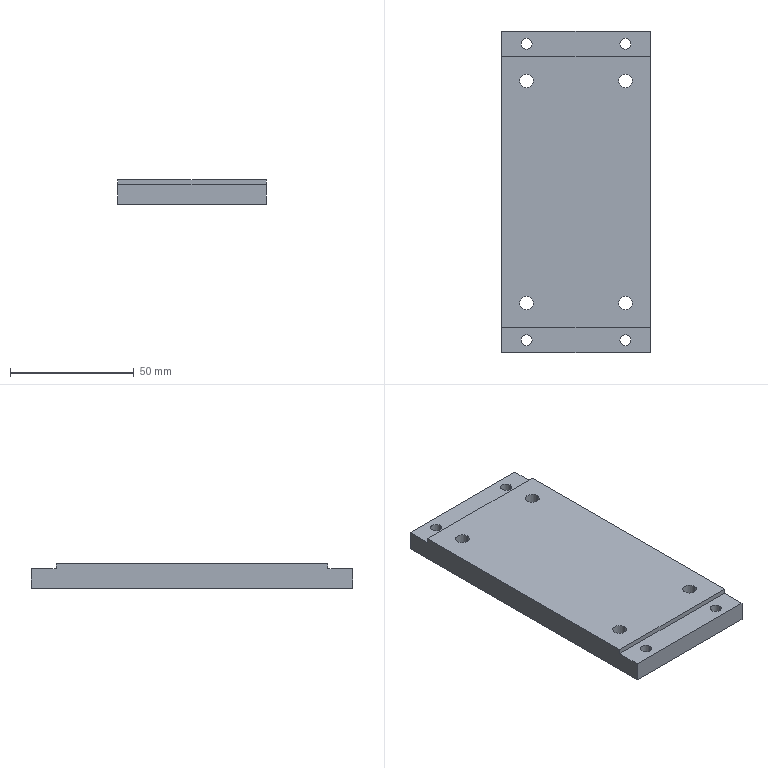Part | SolidWorks | features HoleWzd 2, Extrusion 1, ICE 1 | 1 solid | 38 faces | box 60 x 130 x 10 mm | volume 73508 mm3 | cylinder 24 | plane 14 | commonest cylinder face diameters 4.5 x8 5.5 x8 8 x8
STEP:
#1=CARTESIAN_POINT('',(17.25,45.,0.));
#2=VERTEX_POINT('',#1);
#3=CARTESIAN_POINT('',(22.75,45.,0.));
#4=VERTEX_POINT('',#3);
#5=CARTESIAN_POINT('',(20.,45.,0.));
#6=DIRECTION('',(0.,0.,1.));
#7=DIRECTION('',(1.,0.,0.));
#8=AXIS2_PLACEMENT_3D('',#5,#6,#7);
#9=CIRCLE('',#8,2.75);
#10=EDGE_CURVE('',#2,#4,#9,.T.);
#11=ORIENTED_EDGE('',*,*,#10,.F.);
#12=CARTESIAN_POINT('',(17.25,45.,10.));
#13=VERTEX_POINT('',#12);
#14=CARTESIAN_POINT('',(17.25,45.,10.));
#15=DIRECTION('',(0.,0.,1.));
#16=VECTOR('',#15,1000.);
#17=LINE('',#14,#16);
#18=EDGE_CURVE('',#2,#13,#17,.T.);
#19=ORIENTED_EDGE('',*,*,#18,.T.);
#20=CARTESIAN_POINT('',(22.75,45.,10.));
#21=VERTEX_POINT('',#20);
#22=CARTESIAN_POINT('',(20.,45.,10.));
#23=DIRECTION('',(0.,0.,1.));
#24=DIRECTION('',(1.,0.,0.));
#25=AXIS2_PLACEMENT_3D('',#22,#23,#24);
#26=CIRCLE('',#25,2.75);
#27=EDGE_CURVE('',#13,#21,#26,.T.);
#28=ORIENTED_EDGE('',*,*,#27,.T.);
#29=CARTESIAN_POINT('',(22.75,45.,10.));
#30=DIRECTION('',(0.,0.,1.));
#31=VECTOR('',#30,1000.);
#32=LINE('',#29,#31);
#33=EDGE_CURVE('',#4,#21,#32,.T.);
#34=ORIENTED_EDGE('',*,*,#33,.F.);
#35=EDGE_LOOP('',(#11,#19,#28,#34));
#36=FACE_OUTER_BOUND('',#35,.T.);
#37=CARTESIAN_POINT('',(20.,45.,10.));
#38=DIRECTION('',(0.,0.,1.));
#39=DIRECTION('',(1.,0.,0.));
#40=AXIS2_PLACEMENT_3D('',#37,#38,#39);
#41=CYLINDRICAL_SURFACE('',#40,2.75);
#42=ADVANCED_FACE('',(#36),#41,.F.);
#43=CARTESIAN_POINT('',(17.25,-45.,0.));
#44=VERTEX_POINT('',#43);
#45=CARTESIAN_POINT('',(22.75,-45.,0.));
#46=VERTEX_POINT('',#45);
#47=CARTESIAN_POINT('',(20.,-45.,0.));
#48=DIRECTION('',(0.,0.,1.));
#49=DIRECTION('',(1.,0.,0.));
#50=AXIS2_PLACEMENT_3D('',#47,#48,#49);
#51=CIRCLE('',#50,2.75);
#52=EDGE_CURVE('',#44,#46,#51,.T.);
#53=ORIENTED_EDGE('',*,*,#52,.F.);
#54=CARTESIAN_POINT('',(17.25,-45.,10.));
#55=VERTEX_POINT('',#54);
#56=CARTESIAN_POINT('',(17.25,-45.,10.));
#57=DIRECTION('',(0.,0.,1.));
#58=VECTOR('',#57,1000.);
#59=LINE('',#56,#58);
#60=EDGE_CURVE('',#44,#55,#59,.T.);
#61=ORIENTED_EDGE('',*,*,#60,.T.);
#62=CARTESIAN_POINT('',(22.75,-45.,10.));
#63=VERTEX_POINT('',#62);
#64=CARTESIAN_POINT('',(20.,-45.,10.));
#65=DIRECTION('',(0.,0.,1.));
#66=DIRECTION('',(1.,0.,0.));
#67=AXIS2_PLACEMENT_3D('',#64,#65,#66);
#68=CIRCLE('',#67,2.75);
#69=EDGE_CURVE('',#55,#63,#68,.T.);
#70=ORIENTED_EDGE('',*,*,#69,.T.);
#71=CARTESIAN_POINT('',(22.75,-45.,10.));
#72=DIRECTION('',(0.,0.,1.));
#73=VECTOR('',#72,1000.);
#74=LINE('',#71,#73);
#75=EDGE_CURVE('',#46,#63,#74,.T.);
#76=ORIENTED_EDGE('',*,*,#75,.F.);
#77=EDGE_LOOP('',(#53,#61,#70,#76));
#78=FACE_OUTER_BOUND('',#77,.T.);
#79=CARTESIAN_POINT('',(20.,-45.,10.));
#80=DIRECTION('',(0.,0.,1.));
#81=DIRECTION('',(1.,0.,0.));
#82=AXIS2_PLACEMENT_3D('',#79,#80,#81);
#83=CYLINDRICAL_SURFACE('',#82,2.75);
#84=ADVANCED_FACE('',(#78),#83,.F.);
#85=CARTESIAN_POINT('',(-22.75,45.,0.));
#86=VERTEX_POINT('',#85);
#87=CARTESIAN_POINT('',(-17.25,45.,0.));
#88=VERTEX_POINT('',#87);
#89=CARTESIAN_POINT('',(-20.,45.,0.));
#90=DIRECTION('',(0.,0.,1.));
#91=DIRECTION('',(1.,0.,0.));
#92=AXIS2_PLACEMENT_3D('',#89,#90,#91);
#93=CIRCLE('',#92,2.75);
#94=EDGE_CURVE('',#86,#88,#93,.T.);
#95=ORIENTED_EDGE('',*,*,#94,.F.);
#96=CARTESIAN_POINT('',(-22.75,45.,10.));
#97=VERTEX_POINT('',#96);
#98=CARTESIAN_POINT('',(-22.75,45.,10.));
#99=DIRECTION('',(0.,0.,1.));
#100=VECTOR('',#99,1000.);
#101=LINE('',#98,#100);
#102=EDGE_CURVE('',#86,#97,#101,.T.);
#103=ORIENTED_EDGE('',*,*,#102,.T.);
#104=CARTESIAN_POINT('',(-17.25,45.,10.));
#105=VERTEX_POINT('',#104);
#106=CARTESIAN_POINT('',(-20.,45.,10.));
#107=DIRECTION('',(0.,0.,1.));
#108=DIRECTION('',(1.,0.,0.));
#109=AXIS2_PLACEMENT_3D('',#106,#107,#108);
#110=CIRCLE('',#109,2.75);
#111=EDGE_CURVE('',#97,#105,#110,.T.);
#112=ORIENTED_EDGE('',*,*,#111,.T.);
#113=CARTESIAN_POINT('',(-17.25,45.,10.));
#114=DIRECTION('',(0.,0.,1.));
#115=VECTOR('',#114,1000.);
#116=LINE('',#113,#115);
#117=EDGE_CURVE('',#88,#105,#116,.T.);
#118=ORIENTED_EDGE('',*,*,#117,.F.);
#119=EDGE_LOOP('',(#95,#103,#112,#118));
#120=FACE_OUTER_BOUND('',#119,.T.);
#121=CARTESIAN_POINT('',(-20.,45.,10.));
#122=DIRECTION('',(0.,0.,1.));
#123=DIRECTION('',(1.,0.,0.));
#124=AXIS2_PLACEMENT_3D('',#121,#122,#123);
#125=CYLINDRICAL_SURFACE('',#124,2.75);
#126=ADVANCED_FACE('',(#120),#125,.F.);
#127=CARTESIAN_POINT('',(-22.75,-45.,0.));
#128=VERTEX_POINT('',#127);
#129=CARTESIAN_POINT('',(-17.25,-45.,0.));
#130=VERTEX_POINT('',#129);
#131=CARTESIAN_POINT('',(-20.,-45.,0.));
#132=DIRECTION('',(0.,0.,1.));
#133=DIRECTION('',(1.,0.,0.));
#134=AXIS2_PLACEMENT_3D('',#131,#132,#133);
#135=CIRCLE('',#134,2.75);
#136=EDGE_CURVE('',#128,#130,#135,.T.);
#137=ORIENTED_EDGE('',*,*,#136,.F.);
#138=CARTESIAN_POINT('',(-22.75,-45.,10.));
#139=VERTEX_POINT('',#138);
#140=CARTESIAN_POINT('',(-22.75,-45.,10.));
#141=DIRECTION('',(0.,0.,1.));
#142=VECTOR('',#141,1000.);
#143=LINE('',#140,#142);
#144=EDGE_CURVE('',#128,#139,#143,.T.);
#145=ORIENTED_EDGE('',*,*,#144,.T.);
#146=CARTESIAN_POINT('',(-17.25,-45.,10.));
#147=VERTEX_POINT('',#146);
#148=CARTESIAN_POINT('',(-20.,-45.,10.));
#149=DIRECTION('',(0.,0.,1.));
#150=DIRECTION('',(1.,0.,0.));
#151=AXIS2_PLACEMENT_3D('',#148,#149,#150);
#152=CIRCLE('',#151,2.75);
#153=EDGE_CURVE('',#139,#147,#152,.T.);
#154=ORIENTED_EDGE('',*,*,#153,.T.);
#155=CARTESIAN_POINT('',(-17.25,-45.,10.));
#156=DIRECTION('',(0.,0.,1.));
#157=VECTOR('',#156,1000.);
#158=LINE('',#155,#157);
#159=EDGE_CURVE('',#130,#147,#158,.T.);
#160=ORIENTED_EDGE('',*,*,#159,.F.);
#161=EDGE_LOOP('',(#137,#145,#154,#160));
#162=FACE_OUTER_BOUND('',#161,.T.);
#163=CARTESIAN_POINT('',(-20.,-45.,10.));
#164=DIRECTION('',(0.,0.,1.));
#165=DIRECTION('',(1.,0.,0.));
#166=AXIS2_PLACEMENT_3D('',#163,#164,#165);
#167=CYLINDRICAL_SURFACE('',#166,2.75);
#168=ADVANCED_FACE('',(#162),#167,.F.);
#169=CARTESIAN_POINT('',(-16.,-60.,4.6));
#170=VERTEX_POINT('',#169);
#171=CARTESIAN_POINT('',(-24.,-60.,4.6));
#172=VERTEX_POINT('',#171);
#173=CARTESIAN_POINT('',(-20.,-60.,4.6));
#174=DIRECTION('',(0.,0.,-1.));
#175=DIRECTION('',(-1.,0.,0.));
#176=AXIS2_PLACEMENT_3D('',#173,#174,#175);
#177=CIRCLE('',#176,4.);
#178=EDGE_CURVE('',#170,#172,#177,.T.);
#179=ORIENTED_EDGE('',*,*,#178,.F.);
#180=CARTESIAN_POINT('',(-16.,-60.,0.));
#181=VERTEX_POINT('',#180);
#182=CARTESIAN_POINT('',(-16.,-60.,0.));
#183=DIRECTION('',(0.,0.,-1.));
#184=VECTOR('',#183,1000.);
#185=LINE('',#182,#184);
#186=EDGE_CURVE('',#170,#181,#185,.T.);
#187=ORIENTED_EDGE('',*,*,#186,.T.);
#188=CARTESIAN_POINT('',(-24.,-60.,0.));
#189=VERTEX_POINT('',#188);
#190=CARTESIAN_POINT('',(-20.,-60.,0.));
#191=DIRECTION('',(0.,0.,-1.));
#192=DIRECTION('',(-1.,0.,0.));
#193=AXIS2_PLACEMENT_3D('',#190,#191,#192);
#194=CIRCLE('',#193,4.);
#195=EDGE_CURVE('',#181,#189,#194,.T.);
#196=ORIENTED_EDGE('',*,*,#195,.T.);
#197=CARTESIAN_POINT('',(-24.,-60.,0.));
#198=DIRECTION('',(0.,0.,-1.));
#199=VECTOR('',#198,1000.);
#200=LINE('',#197,#199);
#201=EDGE_CURVE('',#172,#189,#200,.T.);
#202=ORIENTED_EDGE('',*,*,#201,.F.);
#203=EDGE_LOOP('',(#179,#187,#196,#202));
#204=FACE_OUTER_BOUND('',#203,.T.);
#205=CARTESIAN_POINT('',(-20.,-60.,0.));
#206=DIRECTION('',(0.,0.,-1.));
#207=DIRECTION('',(-1.,0.,0.));
#208=AXIS2_PLACEMENT_3D('',#205,#206,#207);
#209=CYLINDRICAL_SURFACE('',#208,4.);
#210=ADVANCED_FACE('',(#204),#209,.F.);
#211=CARTESIAN_POINT('',(-22.25,-60.,8.));
#212=VERTEX_POINT('',#211);
#213=CARTESIAN_POINT('',(-17.75,-60.,8.));
#214=VERTEX_POINT('',#213);
#215=CARTESIAN_POINT('',(-20.,-60.,8.));
#216=DIRECTION('',(0.,0.,1.));
#217=DIRECTION('',(1.,0.,0.));
#218=AXIS2_PLACEMENT_3D('',#215,#216,#217);
#219=CIRCLE('',#218,2.25);
#220=EDGE_CURVE('',#212,#214,#219,.T.);
#221=ORIENTED_EDGE('',*,*,#220,.T.);
#222=CARTESIAN_POINT('',(-17.75,-60.,4.6));
#223=VERTEX_POINT('',#222);
#224=CARTESIAN_POINT('',(-17.75,-60.,0.));
#225=DIRECTION('',(0.,0.,-1.));
#226=VECTOR('',#225,1000.);
#227=LINE('',#224,#226);
#228=EDGE_CURVE('',#214,#223,#227,.T.);
#229=ORIENTED_EDGE('',*,*,#228,.T.);
#230=CARTESIAN_POINT('',(-22.25,-60.,4.6));
#231=VERTEX_POINT('',#230);
#232=CARTESIAN_POINT('',(-20.,-60.,4.6));
#233=DIRECTION('',(0.,0.,-1.));
#234=DIRECTION('',(-1.,0.,0.));
#235=AXIS2_PLACEMENT_3D('',#232,#233,#234);
#236=CIRCLE('',#235,2.25);
#237=EDGE_CURVE('',#223,#231,#236,.T.);
#238=ORIENTED_EDGE('',*,*,#237,.T.);
#239=CARTESIAN_POINT('',(-22.25,-60.,0.));
#240=DIRECTION('',(0.,0.,-1.));
#241=VECTOR('',#240,1000.);
#242=LINE('',#239,#241);
#243=EDGE_CURVE('',#212,#231,#242,.T.);
#244=ORIENTED_EDGE('',*,*,#243,.F.);
#245=EDGE_LOOP('',(#221,#229,#238,#244));
#246=FACE_OUTER_BOUND('',#245,.T.);
#247=CARTESIAN_POINT('',(-20.,-60.,0.));
#248=DIRECTION('',(0.,0.,-1.));
#249=DIRECTION('',(-1.,0.,0.));
#250=AXIS2_PLACEMENT_3D('',#247,#248,#249);
#251=CYLINDRICAL_SURFACE('',#250,2.25);
#252=ADVANCED_FACE('',(#246),#251,.F.);
#253=CARTESIAN_POINT('',(24.,-60.,4.6));
#254=VERTEX_POINT('',#253);
#255=CARTESIAN_POINT('',(16.,-60.,4.6));
#256=VERTEX_POINT('',#255);
#257=CARTESIAN_POINT('',(20.,-60.,4.6));
#258=DIRECTION('',(0.,0.,-1.));
#259=DIRECTION('',(-1.,0.,0.));
#260=AXIS2_PLACEMENT_3D('',#257,#258,#259);
#261=CIRCLE('',#260,4.);
#262=EDGE_CURVE('',#254,#256,#261,.T.);
#263=ORIENTED_EDGE('',*,*,#262,.F.);
#264=CARTESIAN_POINT('',(24.,-60.,0.));
#265=VERTEX_POINT('',#264);
#266=CARTESIAN_POINT('',(24.,-60.,0.));
#267=DIRECTION('',(0.,0.,-1.));
#268=VECTOR('',#267,1000.);
#269=LINE('',#266,#268);
#270=EDGE_CURVE('',#254,#265,#269,.T.);
#271=ORIENTED_EDGE('',*,*,#270,.T.);
#272=CARTESIAN_POINT('',(16.,-60.,0.));
#273=VERTEX_POINT('',#272);
#274=CARTESIAN_POINT('',(20.,-60.,0.));
#275=DIRECTION('',(0.,0.,-1.));
#276=DIRECTION('',(-1.,0.,0.));
#277=AXIS2_PLACEMENT_3D('',#274,#275,#276);
#278=CIRCLE('',#277,4.);
#279=EDGE_CURVE('',#265,#273,#278,.T.);
#280=ORIENTED_EDGE('',*,*,#279,.T.);
#281=CARTESIAN_POINT('',(16.,-60.,0.));
#282=DIRECTION('',(0.,0.,-1.));
#283=VECTOR('',#282,1000.);
#284=LINE('',#281,#283);
#285=EDGE_CURVE('',#256,#273,#284,.T.);
#286=ORIENTED_EDGE('',*,*,#285,.F.);
#287=EDGE_LOOP('',(#263,#271,#280,#286));
#288=FACE_OUTER_BOUND('',#287,.T.);
#289=CARTESIAN_POINT('',(20.,-60.,0.));
#290=DIRECTION('',(0.,0.,-1.));
#291=DIRECTION('',(-1.,0.,0.));
#292=AXIS2_PLACEMENT_3D('',#289,#290,#291);
#293=CYLINDRICAL_SURFACE('',#292,4.);
#294=ADVANCED_FACE('',(#288),#293,.F.);
#295=CARTESIAN_POINT('',(17.75,-60.,8.));
#296=VERTEX_POINT('',#295);
#297=CARTESIAN_POINT('',(22.25,-60.,8.));
#298=VERTEX_POINT('',#297);
#299=CARTESIAN_POINT('',(20.,-60.,8.));
#300=DIRECTION('',(0.,0.,1.));
#301=DIRECTION('',(1.,0.,0.));
#302=AXIS2_PLACEMENT_3D('',#299,#300,#301);
#303=CIRCLE('',#302,2.25);
#304=EDGE_CURVE('',#296,#298,#303,.T.);
#305=ORIENTED_EDGE('',*,*,#304,.T.);
#306=CARTESIAN_POINT('',(22.25,-60.,4.6));
#307=VERTEX_POINT('',#306);
#308=CARTESIAN_POINT('',(22.25,-60.,0.));
#309=DIRECTION('',(0.,0.,-1.));
#310=VECTOR('',#309,1000.);
#311=LINE('',#308,#310);
#312=EDGE_CURVE('',#298,#307,#311,.T.);
#313=ORIENTED_EDGE('',*,*,#312,.T.);
#314=CARTESIAN_POINT('',(17.75,-60.,4.6));
#315=VERTEX_POINT('',#314);
#316=CARTESIAN_POINT('',(20.,-60.,4.6));
#317=DIRECTION('',(0.,0.,-1.));
#318=DIRECTION('',(-1.,0.,0.));
#319=AXIS2_PLACEMENT_3D('',#316,#317,#318);
#320=CIRCLE('',#319,2.25);
#321=EDGE_CURVE('',#307,#315,#320,.T.);
#322=ORIENTED_EDGE('',*,*,#321,.T.);
#323=CARTESIAN_POINT('',(17.75,-60.,0.));
#324=DIRECTION('',(0.,0.,-1.));
#325=VECTOR('',#324,1000.);
#326=LINE('',#323,#325);
#327=EDGE_CURVE('',#296,#315,#326,.T.);
#328=ORIENTED_EDGE('',*,*,#327,.F.);
#329=EDGE_LOOP('',(#305,#313,#322,#328));
#330=FACE_OUTER_BOUND('',#329,.T.);
#331=CARTESIAN_POINT('',(20.,-60.,0.));
#332=DIRECTION('',(0.,0.,-1.));
#333=DIRECTION('',(-1.,0.,0.));
#334=AXIS2_PLACEMENT_3D('',#331,#332,#333);
#335=CYLINDRICAL_SURFACE('',#334,2.25);
#336=ADVANCED_FACE('',(#330),#335,.F.);
#337=CARTESIAN_POINT('',(-16.,60.,4.6));
#338=VERTEX_POINT('',#337);
#339=CARTESIAN_POINT('',(-24.,60.,4.6));
#340=VERTEX_POINT('',#339);
#341=CARTESIAN_POINT('',(-20.,60.,4.6));
#342=DIRECTION('',(0.,0.,-1.));
#343=DIRECTION('',(-1.,0.,0.));
#344=AXIS2_PLACEMENT_3D('',#341,#342,#343);
#345=CIRCLE('',#344,4.);
#346=EDGE_CURVE('',#338,#340,#345,.T.);
#347=ORIENTED_EDGE('',*,*,#346,.F.);
#348=CARTESIAN_POINT('',(-16.,60.,0.));
#349=VERTEX_POINT('',#348);
#350=CARTESIAN_POINT('',(-16.,60.,0.));
#351=DIRECTION('',(0.,0.,-1.));
#352=VECTOR('',#351,1000.);
#353=LINE('',#350,#352);
#354=EDGE_CURVE('',#338,#349,#353,.T.);
#355=ORIENTED_EDGE('',*,*,#354,.T.);
#356=CARTESIAN_POINT('',(-24.,60.,0.));
#357=VERTEX_POINT('',#356);
#358=CARTESIAN_POINT('',(-20.,60.,0.));
#359=DIRECTION('',(0.,0.,-1.));
#360=DIRECTION('',(-1.,0.,0.));
#361=AXIS2_PLACEMENT_3D('',#358,#359,#360);
#362=CIRCLE('',#361,4.);
#363=EDGE_CURVE('',#349,#357,#362,.T.);
#364=ORIENTED_EDGE('',*,*,#363,.T.);
#365=CARTESIAN_POINT('',(-24.,60.,0.));
#366=DIRECTION('',(0.,0.,-1.));
#367=VECTOR('',#366,1000.);
#368=LINE('',#365,#367);
#369=EDGE_CURVE('',#340,#357,#368,.T.);
#370=ORIENTED_EDGE('',*,*,#369,.F.);
#371=EDGE_LOOP('',(#347,#355,#364,#370));
#372=FACE_OUTER_BOUND('',#371,.T.);
#373=CARTESIAN_POINT('',(-20.,60.,0.));
#374=DIRECTION('',(0.,0.,-1.));
#375=DIRECTION('',(-1.,0.,0.));
#376=AXIS2_PLACEMENT_3D('',#373,#374,#375);
#377=CYLINDRICAL_SURFACE('',#376,4.);
#378=ADVANCED_FACE('',(#372),#377,.F.);
#379=CARTESIAN_POINT('',(-22.25,60.,8.));
#380=VERTEX_POINT('',#379);
#381=CARTESIAN_POINT('',(-17.75,60.,8.));
#382=VERTEX_POINT('',#381);
#383=CARTESIAN_POINT('',(-20.,60.,8.));
#384=DIRECTION('',(0.,0.,1.));
#385=DIRECTION('',(1.,0.,0.));
#386=AXIS2_PLACEMENT_3D('',#383,#384,#385);
#387=CIRCLE('',#386,2.25);
#388=EDGE_CURVE('',#380,#382,#387,.T.);
#389=ORIENTED_EDGE('',*,*,#388,.T.);
#390=CARTESIAN_POINT('',(-17.75,60.,4.6));
#391=VERTEX_POINT('',#390);
#392=CARTESIAN_POINT('',(-17.75,60.,0.));
#393=DIRECTION('',(0.,0.,-1.));
#394=VECTOR('',#393,1000.);
#395=LINE('',#392,#394);
#396=EDGE_CURVE('',#382,#391,#395,.T.);
#397=ORIENTED_EDGE('',*,*,#396,.T.);
#398=CARTESIAN_POINT('',(-22.25,60.,4.6));
#399=VERTEX_POINT('',#398);
#400=CARTESIAN_POINT('',(-20.,60.,4.6));
#401=DIRECTION('',(0.,0.,-1.));
#402=DIRECTION('',(-1.,0.,0.));
#403=AXIS2_PLACEMENT_3D('',#400,#401,#402);
#404=CIRCLE('',#403,2.25);
#405=EDGE_CURVE('',#391,#399,#404,.T.);
#406=ORIENTED_EDGE('',*,*,#405,.T.);
#407=CARTESIAN_POINT('',(-22.25,60.,0.));
#408=DIRECTION('',(0.,0.,-1.));
#409=VECTOR('',#408,1000.);
#410=LINE('',#407,#409);
#411=EDGE_CURVE('',#380,#399,#410,.T.);
#412=ORIENTED_EDGE('',*,*,#411,.F.);
#413=EDGE_LOOP('',(#389,#397,#406,#412));
#414=FACE_OUTER_BOUND('',#413,.T.);
#415=CARTESIAN_POINT('',(-20.,60.,0.));
#416=DIRECTION('',(0.,0.,-1.));
#417=DIRECTION('',(-1.,0.,0.));
#418=AXIS2_PLACEMENT_3D('',#415,#416,#417);
#419=CYLINDRICAL_SURFACE('',#418,2.25);
#420=ADVANCED_FACE('',(#414),#419,.F.);
#421=CARTESIAN_POINT('',(24.,60.,4.6));
#422=VERTEX_POINT('',#421);
#423=CARTESIAN_POINT('',(16.,60.,4.6));
#424=VERTEX_POINT('',#423);
#425=CARTESIAN_POINT('',(20.,60.,4.6));
#426=DIRECTION('',(0.,0.,-1.));
#427=DIRECTION('',(-1.,0.,0.));
#428=AXIS2_PLACEMENT_3D('',#425,#426,#427);
#429=CIRCLE('',#428,4.);
#430=EDGE_CURVE('',#422,#424,#429,.T.);
#431=ORIENTED_EDGE('',*,*,#430,.F.);
#432=CARTESIAN_POINT('',(24.,60.,0.));
#433=VERTEX_POINT('',#432);
#434=CARTESIAN_POINT('',(24.,60.,0.));
#435=DIRECTION('',(0.,0.,-1.));
#436=VECTOR('',#435,1000.);
#437=LINE('',#434,#436);
#438=EDGE_CURVE('',#422,#433,#437,.T.);
#439=ORIENTED_EDGE('',*,*,#438,.T.);
#440=CARTESIAN_POINT('',(16.,60.,0.));
#441=VERTEX_POINT('',#440);
#442=CARTESIAN_POINT('',(20.,60.,0.));
#443=DIRECTION('',(0.,0.,-1.));
#444=DIRECTION('',(-1.,0.,0.));
#445=AXIS2_PLACEMENT_3D('',#442,#443,#444);
#446=CIRCLE('',#445,4.);
#447=EDGE_CURVE('',#433,#441,#446,.T.);
#448=ORIENTED_EDGE('',*,*,#447,.T.);
#449=CARTESIAN_POINT('',(16.,60.,0.));
#450=DIRECTION('',(0.,0.,-1.));
#451=VECTOR('',#450,1000.);
#452=LINE('',#449,#451);
#453=EDGE_CURVE('',#424,#441,#452,.T.);
#454=ORIENTED_EDGE('',*,*,#453,.F.);
#455=EDGE_LOOP('',(#431,#439,#448,#454));
#456=FACE_OUTER_BOUND('',#455,.T.);
#457=CARTESIAN_POINT('',(20.,60.,0.));
#458=DIRECTION('',(0.,0.,-1.));
#459=DIRECTION('',(-1.,0.,0.));
#460=AXIS2_PLACEMENT_3D('',#457,#458,#459);
#461=CYLINDRICAL_SURFACE('',#460,4.);
#462=ADVANCED_FACE('',(#456),#461,.F.);
#463=CARTESIAN_POINT('',(17.75,60.,8.));
#464=VERTEX_POINT('',#463);
#465=CARTESIAN_POINT('',(22.25,60.,8.));
#466=VERTEX_POINT('',#465);
#467=CARTESIAN_POINT('',(20.,60.,8.));
#468=DIRECTION('',(0.,0.,1.));
#469=DIRECTION('',(1.,0.,0.));
#470=AXIS2_PLACEMENT_3D('',#467,#468,#469);
#471=CIRCLE('',#470,2.25);
#472=EDGE_CURVE('',#464,#466,#471,.T.);
#473=ORIENTED_EDGE('',*,*,#472,.T.);
#474=CARTESIAN_POINT('',(22.25,60.,4.6));
#475=VERTEX_POINT('',#474);
#476=CARTESIAN_POINT('',(22.25,60.,0.));
#477=DIRECTION('',(0.,0.,-1.));
#478=VECTOR('',#477,1000.);
#479=LINE('',#476,#478);
#480=EDGE_CURVE('',#466,#475,#479,.T.);
#481=ORIENTED_EDGE('',*,*,#480,.T.);
#482=CARTESIAN_POINT('',(17.75,60.,4.6));
#483=VERTEX_POINT('',#482);
#484=CARTESIAN_POINT('',(20.,60.,4.6));
#485=DIRECTION('',(0.,0.,-1.));
#486=DIRECTION('',(-1.,0.,0.));
#487=AXIS2_PLACEMENT_3D('',#484,#485,#486);
#488=CIRCLE('',#487,2.25);
#489=EDGE_CURVE('',#475,#483,#488,.T.);
#490=ORIENTED_EDGE('',*,*,#489,.T.);
#491=CARTESIAN_POINT('',(17.75,60.,0.));
#492=DIRECTION('',(0.,0.,-1.));
#493=VECTOR('',#492,1000.);
#494=LINE('',#491,#493);
#495=EDGE_CURVE('',#464,#483,#494,.T.);
#496=ORIENTED_EDGE('',*,*,#495,.F.);
#497=EDGE_LOOP('',(#473,#481,#490,#496));
#498=FACE_OUTER_BOUND('',#497,.T.);
#499=CARTESIAN_POINT('',(20.,60.,0.));
#500=DIRECTION('',(0.,0.,-1.));
#501=DIRECTION('',(-1.,0.,0.));
#502=AXIS2_PLACEMENT_3D('',#499,#500,#501);
#503=CYLINDRICAL_SURFACE('',#502,2.25);
#504=ADVANCED_FACE('',(#498),#503,.F.);
#505=CARTESIAN_POINT('',(30.,65.,8.));
#506=VERTEX_POINT('',#505);
#507=CARTESIAN_POINT('',(-30.,65.,8.));
#508=VERTEX_POINT('',#507);
#509=CARTESIAN_POINT('',(-30.,65.,8.));
#510=DIRECTION('',(-1.,0.,0.));
#511=VECTOR('',#510,1000.);
#512=LINE('',#509,#511);
#513=EDGE_CURVE('',#506,#508,#512,.T.);
#514=ORIENTED_EDGE('',*,*,#513,.F.);
#515=CARTESIAN_POINT('',(30.,65.,0.));
#516=VERTEX_POINT('',#515);
#517=CARTESIAN_POINT('',(30.,65.,10.));
#518=DIRECTION('',(0.,0.,-1.));
#519=VECTOR('',#518,1000.);
#520=LINE('',#517,#519);
#521=EDGE_CURVE('',#506,#516,#520,.T.);
#522=ORIENTED_EDGE('',*,*,#521,.T.);
#523=CARTESIAN_POINT('',(-30.,65.,0.));
#524=VERTEX_POINT('',#523);
#525=CARTESIAN_POINT('',(-30.,65.,0.));
#526=DIRECTION('',(-1.,0.,0.));
#527=VECTOR('',#526,1000.);
#528=LINE('',#525,#527);
#529=EDGE_CURVE('',#516,#524,#528,.T.);
#530=ORIENTED_EDGE('',*,*,#529,.T.);
#531=CARTESIAN_POINT('',(-30.,65.,10.));
#532=DIRECTION('',(0.,0.,-1.));
#533=VECTOR('',#532,1000.);
#534=LINE('',#531,#533);
#535=EDGE_CURVE('',#508,#524,#534,.T.);
#536=ORIENTED_EDGE('',*,*,#535,.F.);
#537=EDGE_LOOP('',(#514,#522,#530,#536));
#538=FACE_OUTER_BOUND('',#537,.T.);
#539=CARTESIAN_POINT('',(-30.,65.,10.));
#540=DIRECTION('',(0.,-1.,0.));
#541=DIRECTION('',(0.,0.,-1.));
#542=AXIS2_PLACEMENT_3D('',#539,#540,#541);
#543=PLANE('',#542);
#544=ADVANCED_FACE('',(#538),#543,.F.);
#545=CARTESIAN_POINT('',(-30.,-65.,8.));
#546=VERTEX_POINT('',#545);
#547=CARTESIAN_POINT('',(30.,-65.,8.));
#548=VERTEX_POINT('',#547);
#549=CARTESIAN_POINT('',(-30.,-65.,8.));
#550=DIRECTION('',(1.,0.,0.));
#551=VECTOR('',#550,1000.);
#552=LINE('',#549,#551);
#553=EDGE_CURVE('',#546,#548,#552,.T.);
#554=ORIENTED_EDGE('',*,*,#553,.F.);
#555=CARTESIAN_POINT('',(-30.,-65.,0.));
#556=VERTEX_POINT('',#555);
#557=CARTESIAN_POINT('',(-30.,-65.,10.));
#558=DIRECTION('',(0.,0.,-1.));
#559=VECTOR('',#558,1000.);
#560=LINE('',#557,#559);
#561=EDGE_CURVE('',#546,#556,#560,.T.);
#562=ORIENTED_EDGE('',*,*,#561,.T.);
#563=CARTESIAN_POINT('',(30.,-65.,0.));
#564=VERTEX_POINT('',#563);
#565=CARTESIAN_POINT('',(-30.,-65.,0.));
#566=DIRECTION('',(1.,0.,0.));
#567=VECTOR('',#566,1000.);
#568=LINE('',#565,#567);
#569=EDGE_CURVE('',#556,#564,#568,.T.);
#570=ORIENTED_EDGE('',*,*,#569,.T.);
#571=CARTESIAN_POINT('',(30.,-65.,10.));
#572=DIRECTION('',(0.,0.,-1.));
#573=VECTOR('',#572,1000.);
#574=LINE('',#571,#573);
#575=EDGE_CURVE('',#548,#564,#574,.T.);
#576=ORIENTED_EDGE('',*,*,#575,.F.);
#577=EDGE_LOOP('',(#554,#562,#570,#576));
#578=FACE_OUTER_BOUND('',#577,.T.);
#579=CARTESIAN_POINT('',(-30.,-65.,10.));
#580=DIRECTION('',(0.,1.,0.));
#581=DIRECTION('',(0.,0.,1.));
#582=AXIS2_PLACEMENT_3D('',#579,#580,#581);
#583=PLANE('',#582);
#584=ADVANCED_FACE('',(#578),#583,.F.);
#585=CARTESIAN_POINT('',(30.,55.,8.));
#586=VERTEX_POINT('',#585);
#587=CARTESIAN_POINT('',(30.,65.,8.));
#588=DIRECTION('',(0.,1.,0.));
#589=VECTOR('',#588,1000.);
#590=LINE('',#587,#589);
#591=EDGE_CURVE('',#586,#506,#590,.T.);
#592=ORIENTED_EDGE('',*,*,#591,.F.);
#593=CARTESIAN_POINT('',(30.,55.,10.));
#594=VERTEX_POINT('',#593);
#595=CARTESIAN_POINT('',(30.,55.,8.));
#596=DIRECTION('',(0.,0.,1.));
#597=VECTOR('',#596,1000.);
#598=LINE('',#595,#597);
#599=EDGE_CURVE('',#586,#594,#598,.T.);
#600=ORIENTED_EDGE('',*,*,#599,.T.);
#601=CARTESIAN_POINT('',(30.,-55.,10.));
#602=VERTEX_POINT('',#601);
#603=CARTESIAN_POINT('',(30.,65.,10.));
#604=DIRECTION('',(0.,1.,0.));
#605=VECTOR('',#604,1000.);
#606=LINE('',#603,#605);
#607=EDGE_CURVE('',#602,#594,#606,.T.);
#608=ORIENTED_EDGE('',*,*,#607,.F.);
#609=CARTESIAN_POINT('',(30.,-55.,8.));
#610=VERTEX_POINT('',#609);
#611=CARTESIAN_POINT('',(30.,-55.,8.));
#612=DIRECTION('',(0.,0.,1.));
#613=VECTOR('',#612,1000.);
#614=LINE('',#611,#613);
#615=EDGE_CURVE('',#610,#602,#614,.T.);
#616=ORIENTED_EDGE('',*,*,#615,.F.);
#617=CARTESIAN_POINT('',(30.,-65.,8.));
#618=DIRECTION('',(0.,1.,0.));
#619=VECTOR('',#618,1000.);
#620=LINE('',#617,#619);
#621=EDGE_CURVE('',#548,#610,#620,.T.);
#622=ORIENTED_EDGE('',*,*,#621,.F.);
#623=ORIENTED_EDGE('',*,*,#575,.T.);
#624=CARTESIAN_POINT('',(30.,65.,0.));
#625=DIRECTION('',(0.,1.,0.));
#626=VECTOR('',#625,1000.);
#627=LINE('',#624,#626);
#628=EDGE_CURVE('',#564,#516,#627,.T.);
#629=ORIENTED_EDGE('',*,*,#628,.T.);
#630=ORIENTED_EDGE('',*,*,#521,.F.);
#631=EDGE_LOOP('',(#592,#600,#608,#616,#622,#623,#629,#630));
#632=FACE_OUTER_BOUND('',#631,.T.);
#633=CARTESIAN_POINT('',(30.,65.,10.));
#634=DIRECTION('',(-1.,0.,0.));
#635=DIRECTION('',(0.,-1.,0.));
#636=AXIS2_PLACEMENT_3D('',#633,#634,#635);
#637=PLANE('',#636);
#638=ADVANCED_FACE('',(#632),#637,.F.);
#639=CARTESIAN_POINT('',(-30.,55.,10.));
#640=VERTEX_POINT('',#639);
#641=CARTESIAN_POINT('',(-30.,-55.,10.));
#642=VERTEX_POINT('',#641);
#643=CARTESIAN_POINT('',(-30.,65.,10.));
#644=DIRECTION('',(0.,-1.,0.));
#645=VECTOR('',#644,1000.);
#646=LINE('',#643,#645);
#647=EDGE_CURVE('',#640,#642,#646,.T.);
#648=ORIENTED_EDGE('',*,*,#647,.F.);
#649=CARTESIAN_POINT('',(-30.,55.,8.));
#650=VERTEX_POINT('',#649);
#651=CARTESIAN_POINT('',(-30.,55.,8.));
#652=DIRECTION('',(0.,0.,1.));
#653=VECTOR('',#652,1000.);
#654=LINE('',#651,#653);
#655=EDGE_CURVE('',#650,#640,#654,.T.);
#656=ORIENTED_EDGE('',*,*,#655,.F.);
#657=CARTESIAN_POINT('',(-30.,65.,8.));
#658=DIRECTION('',(0.,-1.,0.));
#659=VECTOR('',#658,1000.);
#660=LINE('',#657,#659);
#661=EDGE_CURVE('',#508,#650,#660,.T.);
#662=ORIENTED_EDGE('',*,*,#661,.F.);
#663=ORIENTED_EDGE('',*,*,#535,.T.);
#664=CARTESIAN_POINT('',(-30.,65.,0.));
#665=DIRECTION('',(0.,-1.,0.));
#666=VECTOR('',#665,1000.);
#667=LINE('',#664,#666);
#668=EDGE_CURVE('',#524,#556,#667,.T.);
#669=ORIENTED_EDGE('',*,*,#668,.T.);
#670=ORIENTED_EDGE('',*,*,#561,.F.);
#671=CARTESIAN_POINT('',(-30.,-55.,8.));
#672=VERTEX_POINT('',#671);
#673=CARTESIAN_POINT('',(-30.,-65.,8.));
#674=DIRECTION('',(0.,-1.,0.));
#675=VECTOR('',#674,1000.);
#676=LINE('',#673,#675);
#677=EDGE_CURVE('',#672,#546,#676,.T.);
#678=ORIENTED_EDGE('',*,*,#677,.F.);
#679=CARTESIAN_POINT('',(-30.,-55.,8.));
#680=DIRECTION('',(0.,0.,1.));
#681=VECTOR('',#680,1000.);
#682=LINE('',#679,#681);
#683=EDGE_CURVE('',#672,#642,#682,.T.);
#684=ORIENTED_EDGE('',*,*,#683,.T.);
#685=EDGE_LOOP('',(#648,#656,#662,#663,#669,#670,#678,#684));
#686=FACE_OUTER_BOUND('',#685,.T.);
#687=CARTESIAN_POINT('',(-30.,65.,10.));
#688=DIRECTION('',(1.,0.,0.));
#689=DIRECTION('',(0.,1.,0.));
#690=AXIS2_PLACEMENT_3D('',#687,#688,#689);
#691=PLANE('',#690);
#692=ADVANCED_FACE('',(#686),#691,.F.);
#693=CARTESIAN_POINT('',(20.,45.,10.));
#694=DIRECTION('',(0.,0.,1.));
#695=DIRECTION('',(1.,0.,0.));
#696=AXIS2_PLACEMENT_3D('',#693,#694,#695);
#697=CIRCLE('',#696,2.75);
#698=EDGE_CURVE('',#21,#13,#697,.T.);
#699=ORIENTED_EDGE('',*,*,#698,.F.);
#700=ORIENTED_EDGE('',*,*,#27,.F.);
#701=EDGE_LOOP('',(#699,#700));
#702=FACE_BOUND('',#701,.T.);
#703=CARTESIAN_POINT('',(20.,-45.,10.));
#704=DIRECTION('',(0.,0.,1.));
#705=DIRECTION('',(1.,0.,0.));
#706=AXIS2_PLACEMENT_3D('',#703,#704,#705);
#707=CIRCLE('',#706,2.75);
#708=EDGE_CURVE('',#63,#55,#707,.T.);
#709=ORIENTED_EDGE('',*,*,#708,.F.);
#710=ORIENTED_EDGE('',*,*,#69,.F.);
#711=EDGE_LOOP('',(#709,#710));
#712=FACE_BOUND('',#711,.T.);
#713=CARTESIAN_POINT('',(-20.,45.,10.));
#714=DIRECTION('',(0.,0.,1.));
#715=DIRECTION('',(1.,0.,0.));
#716=AXIS2_PLACEMENT_3D('',#713,#714,#715);
#717=CIRCLE('',#716,2.75);
#718=EDGE_CURVE('',#105,#97,#717,.T.);
#719=ORIENTED_EDGE('',*,*,#718,.F.);
#720=ORIENTED_EDGE('',*,*,#111,.F.);
#721=EDGE_LOOP('',(#719,#720));
#722=FACE_BOUND('',#721,.T.);
#723=CARTESIAN_POINT('',(-20.,-45.,10.));
#724=DIRECTION('',(0.,0.,1.));
#725=DIRECTION('',(1.,0.,0.));
#726=AXIS2_PLACEMENT_3D('',#723,#724,#725);
#727=CIRCLE('',#726,2.75);
#728=EDGE_CURVE('',#147,#139,#727,.T.);
#729=ORIENTED_EDGE('',*,*,#728,.F.);
#730=ORIENTED_EDGE('',*,*,#153,.F.);
#731=EDGE_LOOP('',(#729,#730));
#732=FACE_BOUND('',#731,.T.);
#733=CARTESIAN_POINT('',(-30.,55.,10.));
#734=DIRECTION('',(1.,0.,0.));
#735=VECTOR('',#734,1000.);
#736=LINE('',#733,#735);
#737=EDGE_CURVE('',#640,#594,#736,.T.);
#738=ORIENTED_EDGE('',*,*,#737,.F.);
#739=ORIENTED_EDGE('',*,*,#647,.T.);
#740=CARTESIAN_POINT('',(-30.,-55.,10.));
#741=DIRECTION('',(-1.,0.,0.));
#742=VECTOR('',#741,1000.);
#743=LINE('',#740,#742);
#744=EDGE_CURVE('',#602,#642,#743,.T.);
#745=ORIENTED_EDGE('',*,*,#744,.F.);
#746=ORIENTED_EDGE('',*,*,#607,.T.);
#747=EDGE_LOOP('',(#738,#739,#745,#746));
#748=FACE_OUTER_BOUND('',#747,.T.);
#749=CARTESIAN_POINT('',(0.,0.,10.));
#750=DIRECTION('',(0.,0.,1.));
#751=DIRECTION('',(1.,0.,0.));
#752=AXIS2_PLACEMENT_3D('',#749,#750,#751);
#753=PLANE('',#752);
#754=ADVANCED_FACE('',(#702,#712,#722,#732,#748),#753,.T.);
#755=CARTESIAN_POINT('',(20.,45.,0.));
#756=DIRECTION('',(0.,0.,1.));
#757=DIRECTION('',(1.,0.,0.));
#758=AXIS2_PLACEMENT_3D('',#755,#756,#757);
#759=CIRCLE('',#758,2.75);
#760=EDGE_CURVE('',#4,#2,#759,.T.);
#761=ORIENTED_EDGE('',*,*,#760,.T.);
#762=ORIENTED_EDGE('',*,*,#10,.T.);
#763=EDGE_LOOP('',(#761,#762));
#764=FACE_BOUND('',#763,.T.);
#765=CARTESIAN_POINT('',(20.,-45.,0.));
#766=DIRECTION('',(0.,0.,1.));
#767=DIRECTION('',(1.,0.,0.));
#768=AXIS2_PLACEMENT_3D('',#765,#766,#767);
#769=CIRCLE('',#768,2.75);
#770=EDGE_CURVE('',#46,#44,#769,.T.);
#771=ORIENTED_EDGE('',*,*,#770,.T.);
#772=ORIENTED_EDGE('',*,*,#52,.T.);
#773=EDGE_LOOP('',(#771,#772));
#774=FACE_BOUND('',#773,.T.);
#775=CARTESIAN_POINT('',(-20.,45.,0.));
#776=DIRECTION('',(0.,0.,1.));
#777=DIRECTION('',(1.,0.,0.));
#778=AXIS2_PLACEMENT_3D('',#775,#776,#777);
#779=CIRCLE('',#778,2.75);
#780=EDGE_CURVE('',#88,#86,#779,.T.);
#781=ORIENTED_EDGE('',*,*,#780,.T.);
#782=ORIENTED_EDGE('',*,*,#94,.T.);
#783=EDGE_LOOP('',(#781,#782));
#784=FACE_BOUND('',#783,.T.);
#785=CARTESIAN_POINT('',(-20.,-45.,0.));
#786=DIRECTION('',(0.,0.,1.));
#787=DIRECTION('',(1.,0.,0.));
#788=AXIS2_PLACEMENT_3D('',#785,#786,#787);
#789=CIRCLE('',#788,2.75);
#790=EDGE_CURVE('',#130,#128,#789,.T.);
#791=ORIENTED_EDGE('',*,*,#790,.T.);
#792=ORIENTED_EDGE('',*,*,#136,.T.);
#793=EDGE_LOOP('',(#791,#792));
#794=FACE_BOUND('',#793,.T.);
#795=CARTESIAN_POINT('',(-20.,-60.,0.));
#796=DIRECTION('',(0.,0.,-1.));
#797=DIRECTION('',(-1.,0.,0.));
#798=AXIS2_PLACEMENT_3D('',#795,#796,#797);
#799=CIRCLE('',#798,4.);
#800=EDGE_CURVE('',#189,#181,#799,.T.);
#801=ORIENTED_EDGE('',*,*,#800,.F.);
#802=ORIENTED_EDGE('',*,*,#195,.F.);
#803=EDGE_LOOP('',(#801,#802));
#804=FACE_BOUND('',#803,.T.);
#805=CARTESIAN_POINT('',(20.,-60.,0.));
#806=DIRECTION('',(0.,0.,-1.));
#807=DIRECTION('',(-1.,0.,0.));
#808=AXIS2_PLACEMENT_3D('',#805,#806,#807);
#809=CIRCLE('',#808,4.);
#810=EDGE_CURVE('',#273,#265,#809,.T.);
#811=ORIENTED_EDGE('',*,*,#810,.F.);
#812=ORIENTED_EDGE('',*,*,#279,.F.);
#813=EDGE_LOOP('',(#811,#812));
#814=FACE_BOUND('',#813,.T.);
#815=CARTESIAN_POINT('',(-20.,60.,0.));
#816=DIRECTION('',(0.,0.,-1.));
#817=DIRECTION('',(-1.,0.,0.));
#818=AXIS2_PLACEMENT_3D('',#815,#816,#817);
#819=CIRCLE('',#818,4.);
#820=EDGE_CURVE('',#357,#349,#819,.T.);
#821=ORIENTED_EDGE('',*,*,#820,.F.);
#822=ORIENTED_EDGE('',*,*,#363,.F.);
#823=EDGE_LOOP('',(#821,#822));
#824=FACE_BOUND('',#823,.T.);
#825=CARTESIAN_POINT('',(20.,60.,0.));
#826=DIRECTION('',(0.,0.,-1.));
#827=DIRECTION('',(-1.,0.,0.));
#828=AXIS2_PLACEMENT_3D('',#825,#826,#827);
#829=CIRCLE('',#828,4.);
#830=EDGE_CURVE('',#441,#433,#829,.T.);
#831=ORIENTED_EDGE('',*,*,#830,.F.);
#832=ORIENTED_EDGE('',*,*,#447,.F.);
#833=EDGE_LOOP('',(#831,#832));
#834=FACE_BOUND('',#833,.T.);
#835=ORIENTED_EDGE('',*,*,#628,.F.);
#836=ORIENTED_EDGE('',*,*,#569,.F.);
#837=ORIENTED_EDGE('',*,*,#668,.F.);
#838=ORIENTED_EDGE('',*,*,#529,.F.);
#839=EDGE_LOOP('',(#835,#836,#837,#838));
#840=FACE_OUTER_BOUND('',#839,.T.);
#841=CARTESIAN_POINT('',(0.,0.,0.));
#842=DIRECTION('',(0.,0.,1.));
#843=DIRECTION('',(1.,0.,0.));
#844=AXIS2_PLACEMENT_3D('',#841,#842,#843);
#845=PLANE('',#844);
#846=ADVANCED_FACE('',(#764,#774,#784,#794,#804,#814,#824,#834,#840),#845,.F.);
#847=ORIENTED_EDGE('',*,*,#744,.T.);
#848=ORIENTED_EDGE('',*,*,#683,.F.);
#849=CARTESIAN_POINT('',(-30.,-55.,8.));
#850=DIRECTION('',(-1.,0.,0.));
#851=VECTOR('',#850,1000.);
#852=LINE('',#849,#851);
#853=EDGE_CURVE('',#610,#672,#852,.T.);
#854=ORIENTED_EDGE('',*,*,#853,.F.);
#855=ORIENTED_EDGE('',*,*,#615,.T.);
#856=EDGE_LOOP('',(#847,#848,#854,#855));
#857=FACE_OUTER_BOUND('',#856,.T.);
#858=CARTESIAN_POINT('',(-30.,-55.,8.));
#859=DIRECTION('',(0.,1.,0.));
#860=DIRECTION('',(-1.,0.,0.));
#861=AXIS2_PLACEMENT_3D('',#858,#859,#860);
#862=PLANE('',#861);
#863=ADVANCED_FACE('',(#857),#862,.F.);
#864=ORIENTED_EDGE('',*,*,#220,.F.);
#865=CARTESIAN_POINT('',(-20.,-60.,8.));
#866=DIRECTION('',(0.,0.,1.));
#867=DIRECTION('',(1.,0.,0.));
#868=AXIS2_PLACEMENT_3D('',#865,#866,#867);
#869=CIRCLE('',#868,2.25);
#870=EDGE_CURVE('',#214,#212,#869,.T.);
#871=ORIENTED_EDGE('',*,*,#870,.F.);
#872=EDGE_LOOP('',(#864,#871));
#873=FACE_BOUND('',#872,.T.);
#874=ORIENTED_EDGE('',*,*,#304,.F.);
#875=CARTESIAN_POINT('',(20.,-60.,8.));
#876=DIRECTION('',(0.,0.,1.));
#877=DIRECTION('',(1.,0.,0.));
#878=AXIS2_PLACEMENT_3D('',#875,#876,#877);
#879=CIRCLE('',#878,2.25);
#880=EDGE_CURVE('',#298,#296,#879,.T.);
#881=ORIENTED_EDGE('',*,*,#880,.F.);
#882=EDGE_LOOP('',(#874,#881));
#883=FACE_BOUND('',#882,.T.);
#884=ORIENTED_EDGE('',*,*,#553,.T.);
#885=ORIENTED_EDGE('',*,*,#621,.T.);
#886=ORIENTED_EDGE('',*,*,#853,.T.);
#887=ORIENTED_EDGE('',*,*,#677,.T.);
#888=EDGE_LOOP('',(#884,#885,#886,#887));
#889=FACE_OUTER_BOUND('',#888,.T.);
#890=CARTESIAN_POINT('',(0.,0.,8.));
#891=DIRECTION('',(0.,0.,1.));
#892=DIRECTION('',(1.,0.,0.));
#893=AXIS2_PLACEMENT_3D('',#890,#891,#892);
#894=PLANE('',#893);
#895=ADVANCED_FACE('',(#873,#883,#889),#894,.T.);
#896=ORIENTED_EDGE('',*,*,#737,.T.);
#897=ORIENTED_EDGE('',*,*,#599,.F.);
#898=CARTESIAN_POINT('',(-30.,55.,8.));
#899=DIRECTION('',(1.,0.,0.));
#900=VECTOR('',#899,1000.);
#901=LINE('',#898,#900);
#902=EDGE_CURVE('',#650,#586,#901,.T.);
#903=ORIENTED_EDGE('',*,*,#902,.F.);
#904=ORIENTED_EDGE('',*,*,#655,.T.);
#905=EDGE_LOOP('',(#896,#897,#903,#904));
#906=FACE_OUTER_BOUND('',#905,.T.);
#907=CARTESIAN_POINT('',(-30.,55.,8.));
#908=DIRECTION('',(0.,-1.,0.));
#909=DIRECTION('',(1.,0.,0.));
#910=AXIS2_PLACEMENT_3D('',#907,#908,#909);
#911=PLANE('',#910);
#912=ADVANCED_FACE('',(#906),#911,.F.);
#913=ORIENTED_EDGE('',*,*,#388,.F.);
#914=CARTESIAN_POINT('',(-20.,60.,8.));
#915=DIRECTION('',(0.,0.,1.));
#916=DIRECTION('',(1.,0.,0.));
#917=AXIS2_PLACEMENT_3D('',#914,#915,#916);
#918=CIRCLE('',#917,2.25);
#919=EDGE_CURVE('',#382,#380,#918,.T.);
#920=ORIENTED_EDGE('',*,*,#919,.F.);
#921=EDGE_LOOP('',(#913,#920));
#922=FACE_BOUND('',#921,.T.);
#923=ORIENTED_EDGE('',*,*,#472,.F.);
#924=CARTESIAN_POINT('',(20.,60.,8.));
#925=DIRECTION('',(0.,0.,1.));
#926=DIRECTION('',(1.,0.,0.));
#927=AXIS2_PLACEMENT_3D('',#924,#925,#926);
#928=CIRCLE('',#927,2.25);
#929=EDGE_CURVE('',#466,#464,#928,.T.);
#930=ORIENTED_EDGE('',*,*,#929,.F.);
#931=EDGE_LOOP('',(#923,#930));
#932=FACE_BOUND('',#931,.T.);
#933=ORIENTED_EDGE('',*,*,#661,.T.);
#934=ORIENTED_EDGE('',*,*,#902,.T.);
#935=ORIENTED_EDGE('',*,*,#591,.T.);
#936=ORIENTED_EDGE('',*,*,#513,.T.);
#937=EDGE_LOOP('',(#933,#934,#935,#936));
#938=FACE_OUTER_BOUND('',#937,.T.);
#939=CARTESIAN_POINT('',(0.,0.,8.));
#940=DIRECTION('',(0.,0.,1.));
#941=DIRECTION('',(1.,0.,0.));
#942=AXIS2_PLACEMENT_3D('',#939,#940,#941);
#943=PLANE('',#942);
#944=ADVANCED_FACE('',(#922,#932,#938),#943,.T.);
#945=ORIENTED_EDGE('',*,*,#480,.F.);
#946=ORIENTED_EDGE('',*,*,#929,.T.);
#947=ORIENTED_EDGE('',*,*,#495,.T.);
#948=CARTESIAN_POINT('',(20.,60.,4.6));
#949=DIRECTION('',(0.,0.,-1.));
#950=DIRECTION('',(-1.,0.,0.));
#951=AXIS2_PLACEMENT_3D('',#948,#949,#950);
#952=CIRCLE('',#951,2.25);
#953=EDGE_CURVE('',#483,#475,#952,.T.);
#954=ORIENTED_EDGE('',*,*,#953,.T.);
#955=EDGE_LOOP('',(#945,#946,#947,#954));
#956=FACE_OUTER_BOUND('',#955,.T.);
#957=CARTESIAN_POINT('',(20.,60.,0.));
#958=DIRECTION('',(0.,0.,-1.));
#959=DIRECTION('',(-1.,0.,0.));
#960=AXIS2_PLACEMENT_3D('',#957,#958,#959);
#961=CYLINDRICAL_SURFACE('',#960,2.25);
#962=ADVANCED_FACE('',(#956),#961,.F.);
#963=ORIENTED_EDGE('',*,*,#953,.F.);
#964=ORIENTED_EDGE('',*,*,#489,.F.);
#965=EDGE_LOOP('',(#963,#964));
#966=FACE_BOUND('',#965,.T.);
#967=CARTESIAN_POINT('',(20.,60.,4.6));
#968=DIRECTION('',(0.,0.,-1.));
#969=DIRECTION('',(-1.,0.,0.));
#970=AXIS2_PLACEMENT_3D('',#967,#968,#969);
#971=CIRCLE('',#970,4.);
#972=EDGE_CURVE('',#424,#422,#971,.T.);
#973=ORIENTED_EDGE('',*,*,#972,.T.);
#974=ORIENTED_EDGE('',*,*,#430,.T.);
#975=EDGE_LOOP('',(#973,#974));
#976=FACE_OUTER_BOUND('',#975,.T.);
#977=CARTESIAN_POINT('',(22.25,60.,4.6));
#978=DIRECTION('',(0.,0.,1.));
#979=DIRECTION('',(1.,0.,0.));
#980=AXIS2_PLACEMENT_3D('',#977,#978,#979);
#981=PLANE('',#980);
#982=ADVANCED_FACE('',(#966,#976),#981,.F.);
#983=ORIENTED_EDGE('',*,*,#438,.F.);
#984=ORIENTED_EDGE('',*,*,#972,.F.);
#985=ORIENTED_EDGE('',*,*,#453,.T.);
#986=ORIENTED_EDGE('',*,*,#830,.T.);
#987=EDGE_LOOP('',(#983,#984,#985,#986));
#988=FACE_OUTER_BOUND('',#987,.T.);
#989=CARTESIAN_POINT('',(20.,60.,0.));
#990=DIRECTION('',(0.,0.,-1.));
#991=DIRECTION('',(-1.,0.,0.));
#992=AXIS2_PLACEMENT_3D('',#989,#990,#991);
#993=CYLINDRICAL_SURFACE('',#992,4.);
#994=ADVANCED_FACE('',(#988),#993,.F.);
#995=ORIENTED_EDGE('',*,*,#396,.F.);
#996=ORIENTED_EDGE('',*,*,#919,.T.);
#997=ORIENTED_EDGE('',*,*,#411,.T.);
#998=CARTESIAN_POINT('',(-20.,60.,4.6));
#999=DIRECTION('',(0.,0.,-1.));
#1000=DIRECTION('',(-1.,0.,0.));
#1001=AXIS2_PLACEMENT_3D('',#998,#999,#1000);
#1002=CIRCLE('',#1001,2.25);
#1003=EDGE_CURVE('',#399,#391,#1002,.T.);
#1004=ORIENTED_EDGE('',*,*,#1003,.T.);
#1005=EDGE_LOOP('',(#995,#996,#997,#1004));
#1006=FACE_OUTER_BOUND('',#1005,.T.);
#1007=CARTESIAN_POINT('',(-20.,60.,0.));
#1008=DIRECTION('',(0.,0.,-1.));
#1009=DIRECTION('',(-1.,0.,0.));
#1010=AXIS2_PLACEMENT_3D('',#1007,#1008,#1009);
#1011=CYLINDRICAL_SURFACE('',#1010,2.25);
#1012=ADVANCED_FACE('',(#1006),#1011,.F.);
#1013=ORIENTED_EDGE('',*,*,#1003,.F.);
#1014=ORIENTED_EDGE('',*,*,#405,.F.);
#1015=EDGE_LOOP('',(#1013,#1014));
#1016=FACE_BOUND('',#1015,.T.);
#1017=CARTESIAN_POINT('',(-20.,60.,4.6));
#1018=DIRECTION('',(0.,0.,-1.));
#1019=DIRECTION('',(-1.,0.,0.));
#1020=AXIS2_PLACEMENT_3D('',#1017,#1018,#1019);
#1021=CIRCLE('',#1020,4.);
#1022=EDGE_CURVE('',#340,#338,#1021,.T.);
#1023=ORIENTED_EDGE('',*,*,#1022,.T.);
#1024=ORIENTED_EDGE('',*,*,#346,.T.);
#1025=EDGE_LOOP('',(#1023,#1024));
#1026=FACE_OUTER_BOUND('',#1025,.T.);
#1027=CARTESIAN_POINT('',(-17.75,60.,4.6));
#1028=DIRECTION('',(0.,0.,1.));
#1029=DIRECTION('',(1.,0.,0.));
#1030=AXIS2_PLACEMENT_3D('',#1027,#1028,#1029);
#1031=PLANE('',#1030);
#1032=ADVANCED_FACE('',(#1016,#1026),#1031,.F.);
#1033=ORIENTED_EDGE('',*,*,#354,.F.);
#1034=ORIENTED_EDGE('',*,*,#1022,.F.);
#1035=ORIENTED_EDGE('',*,*,#369,.T.);
#1036=ORIENTED_EDGE('',*,*,#820,.T.);
#1037=EDGE_LOOP('',(#1033,#1034,#1035,#1036));
#1038=FACE_OUTER_BOUND('',#1037,.T.);
#1039=CARTESIAN_POINT('',(-20.,60.,0.));
#1040=DIRECTION('',(0.,0.,-1.));
#1041=DIRECTION('',(-1.,0.,0.));
#1042=AXIS2_PLACEMENT_3D('',#1039,#1040,#1041);
#1043=CYLINDRICAL_SURFACE('',#1042,4.);
#1044=ADVANCED_FACE('',(#1038),#1043,.F.);
#1045=ORIENTED_EDGE('',*,*,#312,.F.);
#1046=ORIENTED_EDGE('',*,*,#880,.T.);
#1047=ORIENTED_EDGE('',*,*,#327,.T.);
#1048=CARTESIAN_POINT('',(20.,-60.,4.6));
#1049=DIRECTION('',(0.,0.,-1.));
#1050=DIRECTION('',(-1.,0.,0.));
#1051=AXIS2_PLACEMENT_3D('',#1048,#1049,#1050);
#1052=CIRCLE('',#1051,2.25);
#1053=EDGE_CURVE('',#315,#307,#1052,.T.);
#1054=ORIENTED_EDGE('',*,*,#1053,.T.);
#1055=EDGE_LOOP('',(#1045,#1046,#1047,#1054));
#1056=FACE_OUTER_BOUND('',#1055,.T.);
#1057=CARTESIAN_POINT('',(20.,-60.,0.));
#1058=DIRECTION('',(0.,0.,-1.));
#1059=DIRECTION('',(-1.,0.,0.));
#1060=AXIS2_PLACEMENT_3D('',#1057,#1058,#1059);
#1061=CYLINDRICAL_SURFACE('',#1060,2.25);
#1062=ADVANCED_FACE('',(#1056),#1061,.F.);
#1063=ORIENTED_EDGE('',*,*,#1053,.F.);
#1064=ORIENTED_EDGE('',*,*,#321,.F.);
#1065=EDGE_LOOP('',(#1063,#1064));
#1066=FACE_BOUND('',#1065,.T.);
#1067=CARTESIAN_POINT('',(20.,-60.,4.6));
#1068=DIRECTION('',(0.,0.,-1.));
#1069=DIRECTION('',(-1.,0.,0.));
#1070=AXIS2_PLACEMENT_3D('',#1067,#1068,#1069);
#1071=CIRCLE('',#1070,4.);
#1072=EDGE_CURVE('',#256,#254,#1071,.T.);
#1073=ORIENTED_EDGE('',*,*,#1072,.T.);
#1074=ORIENTED_EDGE('',*,*,#262,.T.);
#1075=EDGE_LOOP('',(#1073,#1074));
#1076=FACE_OUTER_BOUND('',#1075,.T.);
#1077=CARTESIAN_POINT('',(22.25,-60.,4.6));
#1078=DIRECTION('',(0.,0.,1.));
#1079=DIRECTION('',(1.,0.,0.));
#1080=AXIS2_PLACEMENT_3D('',#1077,#1078,#1079);
#1081=PLANE('',#1080);
#1082=ADVANCED_FACE('',(#1066,#1076),#1081,.F.);
#1083=ORIENTED_EDGE('',*,*,#270,.F.);
#1084=ORIENTED_EDGE('',*,*,#1072,.F.);
#1085=ORIENTED_EDGE('',*,*,#285,.T.);
#1086=ORIENTED_EDGE('',*,*,#810,.T.);
#1087=EDGE_LOOP('',(#1083,#1084,#1085,#1086));
#1088=FACE_OUTER_BOUND('',#1087,.T.);
#1089=CARTESIAN_POINT('',(20.,-60.,0.));
#1090=DIRECTION('',(0.,0.,-1.));
#1091=DIRECTION('',(-1.,0.,0.));
#1092=AXIS2_PLACEMENT_3D('',#1089,#1090,#1091);
#1093=CYLINDRICAL_SURFACE('',#1092,4.);
#1094=ADVANCED_FACE('',(#1088),#1093,.F.);
#1095=ORIENTED_EDGE('',*,*,#228,.F.);
#1096=ORIENTED_EDGE('',*,*,#870,.T.);
#1097=ORIENTED_EDGE('',*,*,#243,.T.);
#1098=CARTESIAN_POINT('',(-20.,-60.,4.6));
#1099=DIRECTION('',(0.,0.,-1.));
#1100=DIRECTION('',(-1.,0.,0.));
#1101=AXIS2_PLACEMENT_3D('',#1098,#1099,#1100);
#1102=CIRCLE('',#1101,2.25);
#1103=EDGE_CURVE('',#231,#223,#1102,.T.);
#1104=ORIENTED_EDGE('',*,*,#1103,.T.);
#1105=EDGE_LOOP('',(#1095,#1096,#1097,#1104));
#1106=FACE_OUTER_BOUND('',#1105,.T.);
#1107=CARTESIAN_POINT('',(-20.,-60.,0.));
#1108=DIRECTION('',(0.,0.,-1.));
#1109=DIRECTION('',(-1.,0.,0.));
#1110=AXIS2_PLACEMENT_3D('',#1107,#1108,#1109);
#1111=CYLINDRICAL_SURFACE('',#1110,2.25);
#1112=ADVANCED_FACE('',(#1106),#1111,.F.);
#1113=ORIENTED_EDGE('',*,*,#1103,.F.);
#1114=ORIENTED_EDGE('',*,*,#237,.F.);
#1115=EDGE_LOOP('',(#1113,#1114));
#1116=FACE_BOUND('',#1115,.T.);
#1117=CARTESIAN_POINT('',(-20.,-60.,4.6));
#1118=DIRECTION('',(0.,0.,-1.));
#1119=DIRECTION('',(-1.,0.,0.));
#1120=AXIS2_PLACEMENT_3D('',#1117,#1118,#1119);
#1121=CIRCLE('',#1120,4.);
#1122=EDGE_CURVE('',#172,#170,#1121,.T.);
#1123=ORIENTED_EDGE('',*,*,#1122,.T.);
#1124=ORIENTED_EDGE('',*,*,#178,.T.);
#1125=EDGE_LOOP('',(#1123,#1124));
#1126=FACE_OUTER_BOUND('',#1125,.T.);
#1127=CARTESIAN_POINT('',(-17.75,-60.,4.6));
#1128=DIRECTION('',(0.,0.,1.));
#1129=DIRECTION('',(1.,0.,0.));
#1130=AXIS2_PLACEMENT_3D('',#1127,#1128,#1129);
#1131=PLANE('',#1130);
#1132=ADVANCED_FACE('',(#1116,#1126),#1131,.F.);
#1133=ORIENTED_EDGE('',*,*,#186,.F.);
#1134=ORIENTED_EDGE('',*,*,#1122,.F.);
#1135=ORIENTED_EDGE('',*,*,#201,.T.);
#1136=ORIENTED_EDGE('',*,*,#800,.T.);
#1137=EDGE_LOOP('',(#1133,#1134,#1135,#1136));
#1138=FACE_OUTER_BOUND('',#1137,.T.);
#1139=CARTESIAN_POINT('',(-20.,-60.,0.));
#1140=DIRECTION('',(0.,0.,-1.));
#1141=DIRECTION('',(-1.,0.,0.));
#1142=AXIS2_PLACEMENT_3D('',#1139,#1140,#1141);
#1143=CYLINDRICAL_SURFACE('',#1142,4.);
#1144=ADVANCED_FACE('',(#1138),#1143,.F.);
#1145=ORIENTED_EDGE('',*,*,#144,.F.);
#1146=ORIENTED_EDGE('',*,*,#790,.F.);
#1147=ORIENTED_EDGE('',*,*,#159,.T.);
#1148=ORIENTED_EDGE('',*,*,#728,.T.);
#1149=EDGE_LOOP('',(#1145,#1146,#1147,#1148));
#1150=FACE_OUTER_BOUND('',#1149,.T.);
#1151=CARTESIAN_POINT('',(-20.,-45.,10.));
#1152=DIRECTION('',(0.,0.,1.));
#1153=DIRECTION('',(1.,0.,0.));
#1154=AXIS2_PLACEMENT_3D('',#1151,#1152,#1153);
#1155=CYLINDRICAL_SURFACE('',#1154,2.75);
#1156=ADVANCED_FACE('',(#1150),#1155,.F.);
#1157=ORIENTED_EDGE('',*,*,#102,.F.);
#1158=ORIENTED_EDGE('',*,*,#780,.F.);
#1159=ORIENTED_EDGE('',*,*,#117,.T.);
#1160=ORIENTED_EDGE('',*,*,#718,.T.);
#1161=EDGE_LOOP('',(#1157,#1158,#1159,#1160));
#1162=FACE_OUTER_BOUND('',#1161,.T.);
#1163=CARTESIAN_POINT('',(-20.,45.,10.));
#1164=DIRECTION('',(0.,0.,1.));
#1165=DIRECTION('',(1.,0.,0.));
#1166=AXIS2_PLACEMENT_3D('',#1163,#1164,#1165);
#1167=CYLINDRICAL_SURFACE('',#1166,2.75);
#1168=ADVANCED_FACE('',(#1162),#1167,.F.);
#1169=ORIENTED_EDGE('',*,*,#60,.F.);
#1170=ORIENTED_EDGE('',*,*,#770,.F.);
#1171=ORIENTED_EDGE('',*,*,#75,.T.);
#1172=ORIENTED_EDGE('',*,*,#708,.T.);
#1173=EDGE_LOOP('',(#1169,#1170,#1171,#1172));
#1174=FACE_OUTER_BOUND('',#1173,.T.);
#1175=CARTESIAN_POINT('',(20.,-45.,10.));
#1176=DIRECTION('',(0.,0.,1.));
#1177=DIRECTION('',(1.,0.,0.));
#1178=AXIS2_PLACEMENT_3D('',#1175,#1176,#1177);
#1179=CYLINDRICAL_SURFACE('',#1178,2.75);
#1180=ADVANCED_FACE('',(#1174),#1179,.F.);
#1181=ORIENTED_EDGE('',*,*,#18,.F.);
#1182=ORIENTED_EDGE('',*,*,#760,.F.);
#1183=ORIENTED_EDGE('',*,*,#33,.T.);
#1184=ORIENTED_EDGE('',*,*,#698,.T.);
#1185=EDGE_LOOP('',(#1181,#1182,#1183,#1184));
#1186=FACE_OUTER_BOUND('',#1185,.T.);
#1187=CARTESIAN_POINT('',(20.,45.,10.));
#1188=DIRECTION('',(0.,0.,1.));
#1189=DIRECTION('',(1.,0.,0.));
#1190=AXIS2_PLACEMENT_3D('',#1187,#1188,#1189);
#1191=CYLINDRICAL_SURFACE('',#1190,2.75);
#1192=ADVANCED_FACE('',(#1186),#1191,.F.);
#1193=CLOSED_SHELL('',(#42,#84,#126,#168,#210,#252,#294,#336,#378,#420,#462,#504,#544,#584,#638,#692,#754,#846,#863,#895,#912,#944,#962,#982,#994,#1012,#1032,#1044,#1062,#1082,#1094,#1112,#1132,#1144,#1156,#1168,#1180,#1192));
#1194=MANIFOLD_SOLID_BREP('',#1193);
#1195=CARTESIAN_POINT('',(0.,0.,0.));
#1196=DIRECTION('',(0.,0.,1.));
#1197=DIRECTION('',(1.,0.,0.));
#1198=AXIS2_PLACEMENT_3D('',#1195,#1196,#1197);
#1199=(LENGTH_UNIT()NAMED_UNIT(*)SI_UNIT(.MILLI.,.METRE.));
#1200=UNCERTAINTY_MEASURE_WITH_UNIT(LENGTH_MEASURE(0.00001),#1199,'','');
#1201=(NAMED_UNIT(*)PLANE_ANGLE_UNIT()SI_UNIT($,.RADIAN.));
#1202=(NAMED_UNIT(*)SI_UNIT($,.STERADIAN.)SOLID_ANGLE_UNIT());
#1203=(GEOMETRIC_REPRESENTATION_CONTEXT(3)GLOBAL_UNCERTAINTY_ASSIGNED_CONTEXT((#1200))GLOBAL_UNIT_ASSIGNED_CONTEXT((#1199,#1201,#1202))REPRESENTATION_CONTEXT('',''));
#1204=ADVANCED_BREP_SHAPE_REPRESENTATION('',(#1194,#1198),#1203);